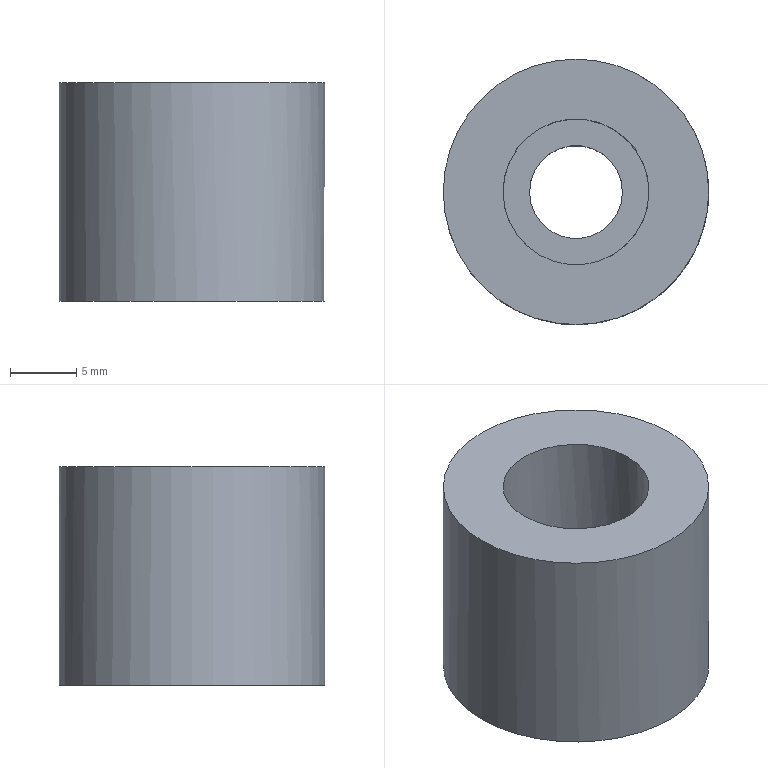Part | NX | features solid 2 | 1 solid | 6 faces | box 20 x 20 x 16.5 mm | volume 4040 mm3 | cylinder 3 | plane 3 | commonest cylinder face diameters 7 x1 11 x1 20 x1
STEP:
#1=CARTESIAN_POINT('',(1685.8,-90.,-16.5));
#2=VERTEX_POINT('',#1);
#3=CARTESIAN_POINT('',(1695.8,-90.,-16.5));
#4=DIRECTION('',(0.,0.,-1.));
#5=DIRECTION('',(-1.,0.,0.));
#6=AXIS2_PLACEMENT_3D('',#3,#4,#5);
#7=CIRCLE('',#6,10.);
#8=EDGE_CURVE('',#2,#2,#7,.T.);
#9=ORIENTED_EDGE('',*,*,#8,.F.);
#10=EDGE_LOOP('',(#9));
#11=FACE_BOUND('',#10,.T.);
#12=CARTESIAN_POINT('',(1705.8,-90.,0.));
#13=VERTEX_POINT('',#12);
#14=CARTESIAN_POINT('',(1695.8,-90.,0.));
#15=DIRECTION('',(0.,0.,1.));
#16=DIRECTION('',(1.,0.,0.));
#17=AXIS2_PLACEMENT_3D('',#14,#15,#16);
#18=CIRCLE('',#17,10.);
#19=EDGE_CURVE('',#13,#13,#18,.T.);
#20=ORIENTED_EDGE('',*,*,#19,.F.);
#21=EDGE_LOOP('',(#20));
#22=FACE_BOUND('',#21,.T.);
#23=CARTESIAN_POINT('',(1695.8,-90.,-16.5));
#24=DIRECTION('',(0.,0.,1.));
#25=DIRECTION('',(-1.,0.,0.));
#26=AXIS2_PLACEMENT_3D('',#23,#24,#25);
#27=CYLINDRICAL_SURFACE('',#26,10.);
#28=ADVANCED_FACE('',(#11,#22),#27,.T.);
#29=CARTESIAN_POINT('',(1690.3,-90.,-9.));
#30=VERTEX_POINT('',#29);
#31=CARTESIAN_POINT('',(1695.8,-90.,-9.));
#32=DIRECTION('',(0.,0.,1.));
#33=DIRECTION('',(-1.,0.,0.));
#34=AXIS2_PLACEMENT_3D('',#31,#32,#33);
#35=CIRCLE('',#34,5.5);
#36=EDGE_CURVE('',#30,#30,#35,.T.);
#37=ORIENTED_EDGE('',*,*,#36,.F.);
#38=EDGE_LOOP('',(#37));
#39=FACE_BOUND('',#38,.T.);
#40=CARTESIAN_POINT('',(1701.3,-90.,0.));
#41=VERTEX_POINT('',#40);
#42=CARTESIAN_POINT('',(1695.8,-90.,0.));
#43=DIRECTION('',(0.,0.,1.));
#44=DIRECTION('',(1.,0.,0.));
#45=AXIS2_PLACEMENT_3D('',#42,#43,#44);
#46=CIRCLE('',#45,5.5);
#47=EDGE_CURVE('',#41,#41,#46,.T.);
#48=ORIENTED_EDGE('',*,*,#47,.T.);
#49=EDGE_LOOP('',(#48));
#50=FACE_BOUND('',#49,.T.);
#51=CARTESIAN_POINT('',(1695.8,-90.,3.5));
#52=DIRECTION('',(0.,0.,-1.));
#53=DIRECTION('',(-1.,0.,0.));
#54=AXIS2_PLACEMENT_3D('',#51,#52,#53);
#55=CYLINDRICAL_SURFACE('',#54,5.5);
#56=ADVANCED_FACE('',(#39,#50),#55,.F.);
#57=ORIENTED_EDGE('',*,*,#8,.T.);
#58=EDGE_LOOP('',(#57));
#59=FACE_BOUND('',#58,.T.);
#60=CARTESIAN_POINT('',(1699.3,-90.,-16.5));
#61=VERTEX_POINT('',#60);
#62=CARTESIAN_POINT('',(1695.8,-90.,-16.5));
#63=DIRECTION('',(0.,0.,-1.));
#64=DIRECTION('',(1.,0.,0.));
#65=AXIS2_PLACEMENT_3D('',#62,#63,#64);
#66=CIRCLE('',#65,3.5);
#67=EDGE_CURVE('',#61,#61,#66,.T.);
#68=ORIENTED_EDGE('',*,*,#67,.F.);
#69=EDGE_LOOP('',(#68));
#70=FACE_BOUND('',#69,.T.);
#71=CARTESIAN_POINT('',(1695.8,-90.,-16.5));
#72=DIRECTION('',(0.,0.,-1.));
#73=DIRECTION('',(1.,0.,0.));
#74=AXIS2_PLACEMENT_3D('',#71,#72,#73);
#75=PLANE('',#74);
#76=ADVANCED_FACE('',(#59,#70),#75,.T.);
#77=CARTESIAN_POINT('',(1692.3,-90.,-9.));
#78=VERTEX_POINT('',#77);
#79=CARTESIAN_POINT('',(1695.8,-90.,-9.));
#80=DIRECTION('',(0.,0.,1.));
#81=DIRECTION('',(-1.,0.,0.));
#82=AXIS2_PLACEMENT_3D('',#79,#80,#81);
#83=CIRCLE('',#82,3.5);
#84=EDGE_CURVE('',#78,#78,#83,.T.);
#85=ORIENTED_EDGE('',*,*,#84,.T.);
#86=EDGE_LOOP('',(#85));
#87=FACE_BOUND('',#86,.T.);
#88=ORIENTED_EDGE('',*,*,#67,.T.);
#89=EDGE_LOOP('',(#88));
#90=FACE_BOUND('',#89,.T.);
#91=CARTESIAN_POINT('',(1695.8,-90.,3.5));
#92=DIRECTION('',(0.,0.,-1.));
#93=DIRECTION('',(-1.,0.,0.));
#94=AXIS2_PLACEMENT_3D('',#91,#92,#93);
#95=CYLINDRICAL_SURFACE('',#94,3.5);
#96=ADVANCED_FACE('',(#87,#90),#95,.F.);
#97=ORIENTED_EDGE('',*,*,#84,.F.);
#98=EDGE_LOOP('',(#97));
#99=FACE_BOUND('',#98,.T.);
#100=ORIENTED_EDGE('',*,*,#36,.T.);
#101=EDGE_LOOP('',(#100));
#102=FACE_BOUND('',#101,.T.);
#103=CARTESIAN_POINT('',(1695.8,-90.,-9.));
#104=DIRECTION('',(0.,0.,-1.));
#105=DIRECTION('',(1.,0.,0.));
#106=AXIS2_PLACEMENT_3D('',#103,#104,#105);
#107=PLANE('',#106);
#108=ADVANCED_FACE('',(#99,#102),#107,.F.);
#109=ORIENTED_EDGE('',*,*,#19,.T.);
#110=EDGE_LOOP('',(#109));
#111=FACE_BOUND('',#110,.T.);
#112=ORIENTED_EDGE('',*,*,#47,.F.);
#113=EDGE_LOOP('',(#112));
#114=FACE_BOUND('',#113,.T.);
#115=CARTESIAN_POINT('',(1658.79,-60.592,0.));
#116=DIRECTION('',(0.,0.,1.));
#117=DIRECTION('',(-1.,0.,0.));
#118=AXIS2_PLACEMENT_3D('',#115,#116,#117);
#119=PLANE('',#118);
#120=ADVANCED_FACE('',(#111,#114),#119,.T.);
#121=CLOSED_SHELL('',(#28,#56,#76,#96,#108,#120));
#122=MANIFOLD_SOLID_BREP('',#121);
#123=(LENGTH_UNIT()NAMED_UNIT(*)SI_UNIT(.MILLI.,.METRE.));
#124=UNCERTAINTY_MEASURE_WITH_UNIT(LENGTH_MEASURE(0.00001),#123,'','');
#125=(NAMED_UNIT(*)PLANE_ANGLE_UNIT()SI_UNIT($,.RADIAN.));
#126=(NAMED_UNIT(*)SI_UNIT($,.STERADIAN.)SOLID_ANGLE_UNIT());
#127=(GEOMETRIC_REPRESENTATION_CONTEXT(3)GLOBAL_UNCERTAINTY_ASSIGNED_CONTEXT((#124))GLOBAL_UNIT_ASSIGNED_CONTEXT((#123,#125,#126))REPRESENTATION_CONTEXT('',''));
#128=ADVANCED_BREP_SHAPE_REPRESENTATION('',(#122),#127);